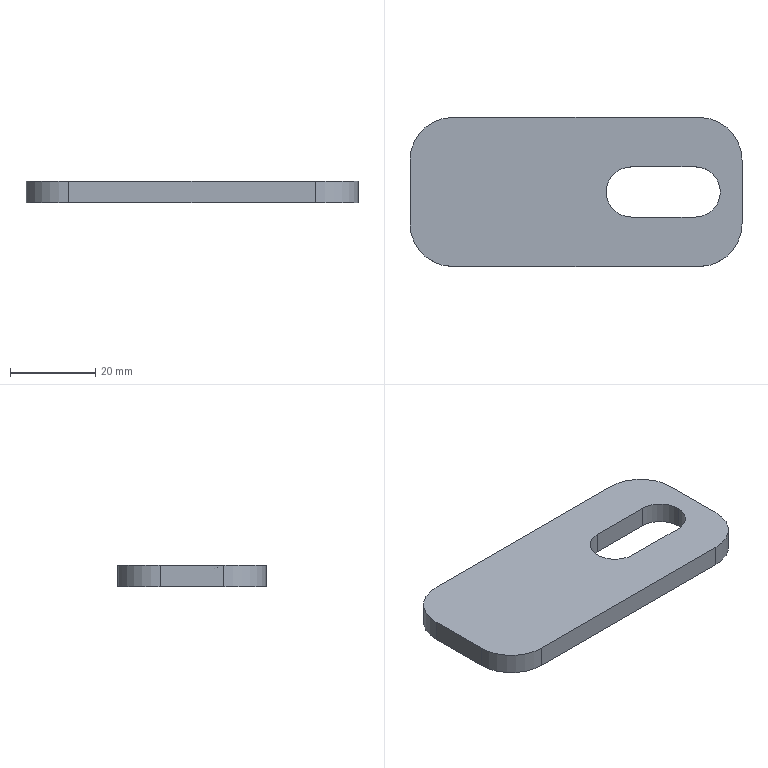Part | SolidWorks | features Fillet 1, FlatPattern 1, SMBaseFlange 1, SheetMetal 1 | 1 solid | 15 faces | box 78 x 35 x 5 mm | volume 11789 mm3 | plane 8 | cylinder 7 | commonest cylinder face diameters 20 x4 11.8 x3
STEP:
#1=CARTESIAN_POINT('',(72.9,-17.5,-5.));
#2=VERTEX_POINT('',#1);
#3=CARTESIAN_POINT('',(67.,-11.6,-5.));
#4=VERTEX_POINT('',#3);
#5=CARTESIAN_POINT('',(67.,-17.5,-5.));
#6=DIRECTION('',(0.,0.,1.));
#7=DIRECTION('',(1.,0.,0.));
#8=AXIS2_PLACEMENT_3D('',#5,#6,#7);
#9=CIRCLE('',#8,5.9);
#10=EDGE_CURVE('',#2,#4,#9,.T.);
#11=ORIENTED_EDGE('',*,*,#10,.F.);
#12=CARTESIAN_POINT('',(72.9,-17.5,0.));
#13=VERTEX_POINT('',#12);
#14=CARTESIAN_POINT('',(72.9,-17.5,-5.));
#15=DIRECTION('',(0.,0.,1.));
#16=VECTOR('',#15,1000.);
#17=LINE('',#14,#16);
#18=EDGE_CURVE('',#2,#13,#17,.T.);
#19=ORIENTED_EDGE('',*,*,#18,.T.);
#20=CARTESIAN_POINT('',(67.,-11.6,0.));
#21=VERTEX_POINT('',#20);
#22=CARTESIAN_POINT('',(67.,-17.5,0.));
#23=DIRECTION('',(0.,0.,1.));
#24=DIRECTION('',(1.,0.,0.));
#25=AXIS2_PLACEMENT_3D('',#22,#23,#24);
#26=CIRCLE('',#25,5.9);
#27=EDGE_CURVE('',#13,#21,#26,.T.);
#28=ORIENTED_EDGE('',*,*,#27,.T.);
#29=CARTESIAN_POINT('',(67.,-11.6,-5.));
#30=DIRECTION('',(0.,0.,1.));
#31=VECTOR('',#30,1000.);
#32=LINE('',#29,#31);
#33=EDGE_CURVE('',#4,#21,#32,.T.);
#34=ORIENTED_EDGE('',*,*,#33,.F.);
#35=EDGE_LOOP('',(#11,#19,#28,#34));
#36=FACE_OUTER_BOUND('',#35,.T.);
#37=CARTESIAN_POINT('',(67.,-17.5,-5.));
#38=DIRECTION('',(0.,0.,1.));
#39=DIRECTION('',(1.,0.,0.));
#40=AXIS2_PLACEMENT_3D('',#37,#38,#39);
#41=CYLINDRICAL_SURFACE('',#40,5.9);
#42=ADVANCED_FACE('',(#36),#41,.F.);
#43=CARTESIAN_POINT('',(0.,-10.,-5.));
#44=VERTEX_POINT('',#43);
#45=CARTESIAN_POINT('',(0.,-25.,-5.));
#46=VERTEX_POINT('',#45);
#47=CARTESIAN_POINT('',(0.,0.,-5.));
#48=DIRECTION('',(0.,-1.,0.));
#49=VECTOR('',#48,1000.);
#50=LINE('',#47,#49);
#51=EDGE_CURVE('',#44,#46,#50,.T.);
#52=ORIENTED_EDGE('',*,*,#51,.T.);
#53=CARTESIAN_POINT('',(0.,-25.,0.));
#54=VERTEX_POINT('',#53);
#55=CARTESIAN_POINT('',(0.,-25.,-5.));
#56=DIRECTION('',(0.,0.,1.));
#57=VECTOR('',#56,1000.);
#58=LINE('',#55,#57);
#59=EDGE_CURVE('',#46,#54,#58,.T.);
#60=ORIENTED_EDGE('',*,*,#59,.T.);
#61=CARTESIAN_POINT('',(0.,-10.,0.));
#62=VERTEX_POINT('',#61);
#63=CARTESIAN_POINT('',(0.,0.,0.));
#64=DIRECTION('',(0.,-1.,0.));
#65=VECTOR('',#64,1000.);
#66=LINE('',#63,#65);
#67=EDGE_CURVE('',#62,#54,#66,.T.);
#68=ORIENTED_EDGE('',*,*,#67,.F.);
#69=CARTESIAN_POINT('',(0.,-10.,-5.));
#70=DIRECTION('',(0.,0.,-1.));
#71=VECTOR('',#70,1000.);
#72=LINE('',#69,#71);
#73=EDGE_CURVE('',#62,#44,#72,.T.);
#74=ORIENTED_EDGE('',*,*,#73,.T.);
#75=EDGE_LOOP('',(#52,#60,#68,#74));
#76=FACE_OUTER_BOUND('',#75,.T.);
#77=CARTESIAN_POINT('',(0.,0.,-5.));
#78=DIRECTION('',(-1.,0.,0.));
#79=DIRECTION('',(0.,-1.,0.));
#80=AXIS2_PLACEMENT_3D('',#77,#78,#79);
#81=PLANE('',#80);
#82=ADVANCED_FACE('',(#76),#81,.T.);
#83=CARTESIAN_POINT('',(68.,0.,0.));
#84=VERTEX_POINT('',#83);
#85=CARTESIAN_POINT('',(10.,0.,0.));
#86=VERTEX_POINT('',#85);
#87=CARTESIAN_POINT('',(0.,0.,0.));
#88=DIRECTION('',(-1.,0.,0.));
#89=VECTOR('',#88,1000.);
#90=LINE('',#87,#89);
#91=EDGE_CURVE('',#84,#86,#90,.T.);
#92=ORIENTED_EDGE('',*,*,#91,.F.);
#93=CARTESIAN_POINT('',(68.,0.,-5.));
#94=VERTEX_POINT('',#93);
#95=CARTESIAN_POINT('',(68.,0.,-5.));
#96=DIRECTION('',(0.,0.,-1.));
#97=VECTOR('',#96,1000.);
#98=LINE('',#95,#97);
#99=EDGE_CURVE('',#84,#94,#98,.T.);
#100=ORIENTED_EDGE('',*,*,#99,.T.);
#101=CARTESIAN_POINT('',(10.,0.,-5.));
#102=VERTEX_POINT('',#101);
#103=CARTESIAN_POINT('',(0.,0.,-5.));
#104=DIRECTION('',(-1.,0.,0.));
#105=VECTOR('',#104,1000.);
#106=LINE('',#103,#105);
#107=EDGE_CURVE('',#94,#102,#106,.T.);
#108=ORIENTED_EDGE('',*,*,#107,.T.);
#109=CARTESIAN_POINT('',(10.,0.,-5.));
#110=DIRECTION('',(0.,0.,1.));
#111=VECTOR('',#110,1000.);
#112=LINE('',#109,#111);
#113=EDGE_CURVE('',#102,#86,#112,.T.);
#114=ORIENTED_EDGE('',*,*,#113,.T.);
#115=EDGE_LOOP('',(#92,#100,#108,#114));
#116=FACE_OUTER_BOUND('',#115,.T.);
#117=CARTESIAN_POINT('',(0.,0.,-5.));
#118=DIRECTION('',(0.,1.,0.));
#119=DIRECTION('',(0.,0.,1.));
#120=AXIS2_PLACEMENT_3D('',#117,#118,#119);
#121=PLANE('',#120);
#122=ADVANCED_FACE('',(#116),#121,.T.);
#123=CARTESIAN_POINT('',(78.,-25.,-5.));
#124=VERTEX_POINT('',#123);
#125=CARTESIAN_POINT('',(78.,-10.,-5.));
#126=VERTEX_POINT('',#125);
#127=CARTESIAN_POINT('',(78.,0.,-5.));
#128=DIRECTION('',(0.,1.,0.));
#129=VECTOR('',#128,1000.);
#130=LINE('',#127,#129);
#131=EDGE_CURVE('',#124,#126,#130,.T.);
#132=ORIENTED_EDGE('',*,*,#131,.T.);
#133=CARTESIAN_POINT('',(78.,-10.,0.));
#134=VERTEX_POINT('',#133);
#135=CARTESIAN_POINT('',(78.,-10.,-5.));
#136=DIRECTION('',(0.,0.,1.));
#137=VECTOR('',#136,1000.);
#138=LINE('',#135,#137);
#139=EDGE_CURVE('',#126,#134,#138,.T.);
#140=ORIENTED_EDGE('',*,*,#139,.T.);
#141=CARTESIAN_POINT('',(78.,-25.,0.));
#142=VERTEX_POINT('',#141);
#143=CARTESIAN_POINT('',(78.,0.,0.));
#144=DIRECTION('',(0.,1.,0.));
#145=VECTOR('',#144,1000.);
#146=LINE('',#143,#145);
#147=EDGE_CURVE('',#142,#134,#146,.T.);
#148=ORIENTED_EDGE('',*,*,#147,.F.);
#149=CARTESIAN_POINT('',(78.,-25.,-5.));
#150=DIRECTION('',(0.,0.,-1.));
#151=VECTOR('',#150,1000.);
#152=LINE('',#149,#151);
#153=EDGE_CURVE('',#142,#124,#152,.T.);
#154=ORIENTED_EDGE('',*,*,#153,.T.);
#155=EDGE_LOOP('',(#132,#140,#148,#154));
#156=FACE_OUTER_BOUND('',#155,.T.);
#157=CARTESIAN_POINT('',(78.,0.,-5.));
#158=DIRECTION('',(1.,0.,0.));
#159=DIRECTION('',(0.,0.,-1.));
#160=AXIS2_PLACEMENT_3D('',#157,#158,#159);
#161=PLANE('',#160);
#162=ADVANCED_FACE('',(#156),#161,.T.);
#163=CARTESIAN_POINT('',(10.,-35.,-5.));
#164=VERTEX_POINT('',#163);
#165=CARTESIAN_POINT('',(68.,-35.,-5.));
#166=VERTEX_POINT('',#165);
#167=CARTESIAN_POINT('',(0.,-35.,-5.));
#168=DIRECTION('',(1.,0.,0.));
#169=VECTOR('',#168,1000.);
#170=LINE('',#167,#169);
#171=EDGE_CURVE('',#164,#166,#170,.T.);
#172=ORIENTED_EDGE('',*,*,#171,.T.);
#173=CARTESIAN_POINT('',(68.,-35.,0.));
#174=VERTEX_POINT('',#173);
#175=CARTESIAN_POINT('',(68.,-35.,-5.));
#176=DIRECTION('',(0.,0.,1.));
#177=VECTOR('',#176,1000.);
#178=LINE('',#175,#177);
#179=EDGE_CURVE('',#166,#174,#178,.T.);
#180=ORIENTED_EDGE('',*,*,#179,.T.);
#181=CARTESIAN_POINT('',(10.,-35.,0.));
#182=VERTEX_POINT('',#181);
#183=CARTESIAN_POINT('',(0.,-35.,0.));
#184=DIRECTION('',(1.,0.,0.));
#185=VECTOR('',#184,1000.);
#186=LINE('',#183,#185);
#187=EDGE_CURVE('',#182,#174,#186,.T.);
#188=ORIENTED_EDGE('',*,*,#187,.F.);
#189=CARTESIAN_POINT('',(10.,-35.,-5.));
#190=DIRECTION('',(0.,0.,-1.));
#191=VECTOR('',#190,1000.);
#192=LINE('',#189,#191);
#193=EDGE_CURVE('',#182,#164,#192,.T.);
#194=ORIENTED_EDGE('',*,*,#193,.T.);
#195=EDGE_LOOP('',(#172,#180,#188,#194));
#196=FACE_OUTER_BOUND('',#195,.T.);
#197=CARTESIAN_POINT('',(0.,-35.,-5.));
#198=DIRECTION('',(0.,-1.,0.));
#199=DIRECTION('',(0.,0.,-1.));
#200=AXIS2_PLACEMENT_3D('',#197,#198,#199);
#201=PLANE('',#200);
#202=ADVANCED_FACE('',(#196),#201,.T.);
#203=CARTESIAN_POINT('',(52.,-23.4,-5.));
#204=VERTEX_POINT('',#203);
#205=CARTESIAN_POINT('',(67.,-23.4,-5.));
#206=VERTEX_POINT('',#205);
#207=CARTESIAN_POINT('',(67.,-23.4,-5.));
#208=DIRECTION('',(1.,0.,0.));
#209=VECTOR('',#208,1000.);
#210=LINE('',#207,#209);
#211=EDGE_CURVE('',#204,#206,#210,.T.);
#212=ORIENTED_EDGE('',*,*,#211,.T.);
#213=CARTESIAN_POINT('',(67.,-17.5,-5.));
#214=DIRECTION('',(0.,0.,1.));
#215=DIRECTION('',(1.,0.,0.));
#216=AXIS2_PLACEMENT_3D('',#213,#214,#215);
#217=CIRCLE('',#216,5.9);
#218=EDGE_CURVE('',#206,#2,#217,.T.);
#219=ORIENTED_EDGE('',*,*,#218,.T.);
#220=ORIENTED_EDGE('',*,*,#10,.T.);
#221=CARTESIAN_POINT('',(52.,-11.6,-5.));
#222=VERTEX_POINT('',#221);
#223=CARTESIAN_POINT('',(67.,-11.6,-5.));
#224=DIRECTION('',(-1.,0.,0.));
#225=VECTOR('',#224,1000.);
#226=LINE('',#223,#225);
#227=EDGE_CURVE('',#4,#222,#226,.T.);
#228=ORIENTED_EDGE('',*,*,#227,.T.);
#229=CARTESIAN_POINT('',(52.,-17.5,-5.));
#230=DIRECTION('',(0.,0.,1.));
#231=DIRECTION('',(1.,0.,0.));
#232=AXIS2_PLACEMENT_3D('',#229,#230,#231);
#233=CIRCLE('',#232,5.9);
#234=EDGE_CURVE('',#222,#204,#233,.T.);
#235=ORIENTED_EDGE('',*,*,#234,.T.);
#236=EDGE_LOOP('',(#212,#219,#220,#228,#235));
#237=FACE_BOUND('',#236,.T.);
#238=ORIENTED_EDGE('',*,*,#107,.F.);
#239=CARTESIAN_POINT('',(68.,-10.,-5.));
#240=DIRECTION('',(0.,0.,-1.));
#241=DIRECTION('',(1.,0.,0.));
#242=AXIS2_PLACEMENT_3D('',#239,#240,#241);
#243=CIRCLE('',#242,10.);
#244=EDGE_CURVE('',#94,#126,#243,.T.);
#245=ORIENTED_EDGE('',*,*,#244,.T.);
#246=ORIENTED_EDGE('',*,*,#131,.F.);
#247=CARTESIAN_POINT('',(68.,-25.,-5.));
#248=DIRECTION('',(0.,0.,-1.));
#249=DIRECTION('',(1.,0.,0.));
#250=AXIS2_PLACEMENT_3D('',#247,#248,#249);
#251=CIRCLE('',#250,10.);
#252=EDGE_CURVE('',#124,#166,#251,.T.);
#253=ORIENTED_EDGE('',*,*,#252,.T.);
#254=ORIENTED_EDGE('',*,*,#171,.F.);
#255=CARTESIAN_POINT('',(10.,-25.,-5.));
#256=DIRECTION('',(0.,0.,-1.));
#257=DIRECTION('',(1.,0.,0.));
#258=AXIS2_PLACEMENT_3D('',#255,#256,#257);
#259=CIRCLE('',#258,10.);
#260=EDGE_CURVE('',#164,#46,#259,.T.);
#261=ORIENTED_EDGE('',*,*,#260,.T.);
#262=ORIENTED_EDGE('',*,*,#51,.F.);
#263=CARTESIAN_POINT('',(10.,-10.,-5.));
#264=DIRECTION('',(0.,0.,-1.));
#265=DIRECTION('',(1.,0.,0.));
#266=AXIS2_PLACEMENT_3D('',#263,#264,#265);
#267=CIRCLE('',#266,10.);
#268=EDGE_CURVE('',#44,#102,#267,.T.);
#269=ORIENTED_EDGE('',*,*,#268,.T.);
#270=EDGE_LOOP('',(#238,#245,#246,#253,#254,#261,#262,#269));
#271=FACE_OUTER_BOUND('',#270,.T.);
#272=CARTESIAN_POINT('',(0.,0.,-5.));
#273=DIRECTION('',(0.,0.,1.));
#274=DIRECTION('',(1.,0.,0.));
#275=AXIS2_PLACEMENT_3D('',#272,#273,#274);
#276=PLANE('',#275);
#277=ADVANCED_FACE('',(#237,#271),#276,.F.);
#278=CARTESIAN_POINT('',(67.,-23.4,0.));
#279=VERTEX_POINT('',#278);
#280=CARTESIAN_POINT('',(67.,-17.5,0.));
#281=DIRECTION('',(0.,0.,1.));
#282=DIRECTION('',(1.,0.,0.));
#283=AXIS2_PLACEMENT_3D('',#280,#281,#282);
#284=CIRCLE('',#283,5.9);
#285=EDGE_CURVE('',#279,#13,#284,.T.);
#286=ORIENTED_EDGE('',*,*,#285,.F.);
#287=CARTESIAN_POINT('',(52.,-23.4,0.));
#288=VERTEX_POINT('',#287);
#289=CARTESIAN_POINT('',(67.,-23.4,0.));
#290=DIRECTION('',(1.,0.,0.));
#291=VECTOR('',#290,1000.);
#292=LINE('',#289,#291);
#293=EDGE_CURVE('',#288,#279,#292,.T.);
#294=ORIENTED_EDGE('',*,*,#293,.F.);
#295=CARTESIAN_POINT('',(52.,-11.6,0.));
#296=VERTEX_POINT('',#295);
#297=CARTESIAN_POINT('',(52.,-17.5,0.));
#298=DIRECTION('',(0.,0.,1.));
#299=DIRECTION('',(1.,0.,0.));
#300=AXIS2_PLACEMENT_3D('',#297,#298,#299);
#301=CIRCLE('',#300,5.9);
#302=EDGE_CURVE('',#296,#288,#301,.T.);
#303=ORIENTED_EDGE('',*,*,#302,.F.);
#304=CARTESIAN_POINT('',(67.,-11.6,0.));
#305=DIRECTION('',(-1.,0.,0.));
#306=VECTOR('',#305,1000.);
#307=LINE('',#304,#306);
#308=EDGE_CURVE('',#21,#296,#307,.T.);
#309=ORIENTED_EDGE('',*,*,#308,.F.);
#310=ORIENTED_EDGE('',*,*,#27,.F.);
#311=EDGE_LOOP('',(#286,#294,#303,#309,#310));
#312=FACE_BOUND('',#311,.T.);
#313=ORIENTED_EDGE('',*,*,#147,.T.);
#314=CARTESIAN_POINT('',(68.,-10.,0.));
#315=DIRECTION('',(0.,0.,1.));
#316=DIRECTION('',(1.,0.,0.));
#317=AXIS2_PLACEMENT_3D('',#314,#315,#316);
#318=CIRCLE('',#317,10.);
#319=EDGE_CURVE('',#134,#84,#318,.T.);
#320=ORIENTED_EDGE('',*,*,#319,.T.);
#321=ORIENTED_EDGE('',*,*,#91,.T.);
#322=CARTESIAN_POINT('',(10.,-10.,0.));
#323=DIRECTION('',(0.,0.,1.));
#324=DIRECTION('',(1.,0.,0.));
#325=AXIS2_PLACEMENT_3D('',#322,#323,#324);
#326=CIRCLE('',#325,10.);
#327=EDGE_CURVE('',#86,#62,#326,.T.);
#328=ORIENTED_EDGE('',*,*,#327,.T.);
#329=ORIENTED_EDGE('',*,*,#67,.T.);
#330=CARTESIAN_POINT('',(10.,-25.,0.));
#331=DIRECTION('',(0.,0.,1.));
#332=DIRECTION('',(1.,0.,0.));
#333=AXIS2_PLACEMENT_3D('',#330,#331,#332);
#334=CIRCLE('',#333,10.);
#335=EDGE_CURVE('',#54,#182,#334,.T.);
#336=ORIENTED_EDGE('',*,*,#335,.T.);
#337=ORIENTED_EDGE('',*,*,#187,.T.);
#338=CARTESIAN_POINT('',(68.,-25.,0.));
#339=DIRECTION('',(0.,0.,1.));
#340=DIRECTION('',(1.,0.,0.));
#341=AXIS2_PLACEMENT_3D('',#338,#339,#340);
#342=CIRCLE('',#341,10.);
#343=EDGE_CURVE('',#174,#142,#342,.T.);
#344=ORIENTED_EDGE('',*,*,#343,.T.);
#345=EDGE_LOOP('',(#313,#320,#321,#328,#329,#336,#337,#344));
#346=FACE_OUTER_BOUND('',#345,.T.);
#347=CARTESIAN_POINT('',(0.,0.,0.));
#348=DIRECTION('',(0.,0.,1.));
#349=DIRECTION('',(1.,0.,0.));
#350=AXIS2_PLACEMENT_3D('',#347,#348,#349);
#351=PLANE('',#350);
#352=ADVANCED_FACE('',(#312,#346),#351,.T.);
#353=ORIENTED_EDGE('',*,*,#18,.F.);
#354=ORIENTED_EDGE('',*,*,#218,.F.);
#355=CARTESIAN_POINT('',(67.,-23.4,-5.));
#356=DIRECTION('',(0.,0.,1.));
#357=VECTOR('',#356,1000.);
#358=LINE('',#355,#357);
#359=EDGE_CURVE('',#206,#279,#358,.T.);
#360=ORIENTED_EDGE('',*,*,#359,.T.);
#361=ORIENTED_EDGE('',*,*,#285,.T.);
#362=EDGE_LOOP('',(#353,#354,#360,#361));
#363=FACE_OUTER_BOUND('',#362,.T.);
#364=CARTESIAN_POINT('',(67.,-17.5,-5.));
#365=DIRECTION('',(0.,0.,1.));
#366=DIRECTION('',(1.,0.,0.));
#367=AXIS2_PLACEMENT_3D('',#364,#365,#366);
#368=CYLINDRICAL_SURFACE('',#367,5.9);
#369=ADVANCED_FACE('',(#363),#368,.F.);
#370=ORIENTED_EDGE('',*,*,#293,.T.);
#371=ORIENTED_EDGE('',*,*,#359,.F.);
#372=ORIENTED_EDGE('',*,*,#211,.F.);
#373=CARTESIAN_POINT('',(52.,-23.4,-5.));
#374=DIRECTION('',(0.,0.,1.));
#375=VECTOR('',#374,1000.);
#376=LINE('',#373,#375);
#377=EDGE_CURVE('',#204,#288,#376,.T.);
#378=ORIENTED_EDGE('',*,*,#377,.T.);
#379=EDGE_LOOP('',(#370,#371,#372,#378));
#380=FACE_OUTER_BOUND('',#379,.T.);
#381=CARTESIAN_POINT('',(67.,-23.4,-5.));
#382=DIRECTION('',(0.,-1.,0.));
#383=DIRECTION('',(0.,0.,-1.));
#384=AXIS2_PLACEMENT_3D('',#381,#382,#383);
#385=PLANE('',#384);
#386=ADVANCED_FACE('',(#380),#385,.F.);
#387=ORIENTED_EDGE('',*,*,#302,.T.);
#388=ORIENTED_EDGE('',*,*,#377,.F.);
#389=ORIENTED_EDGE('',*,*,#234,.F.);
#390=CARTESIAN_POINT('',(52.,-11.6,-5.));
#391=DIRECTION('',(0.,0.,1.));
#392=VECTOR('',#391,1000.);
#393=LINE('',#390,#392);
#394=EDGE_CURVE('',#222,#296,#393,.T.);
#395=ORIENTED_EDGE('',*,*,#394,.T.);
#396=EDGE_LOOP('',(#387,#388,#389,#395));
#397=FACE_OUTER_BOUND('',#396,.T.);
#398=CARTESIAN_POINT('',(52.,-17.5,-5.));
#399=DIRECTION('',(0.,0.,1.));
#400=DIRECTION('',(1.,0.,0.));
#401=AXIS2_PLACEMENT_3D('',#398,#399,#400);
#402=CYLINDRICAL_SURFACE('',#401,5.9);
#403=ADVANCED_FACE('',(#397),#402,.F.);
#404=ORIENTED_EDGE('',*,*,#308,.T.);
#405=ORIENTED_EDGE('',*,*,#394,.F.);
#406=ORIENTED_EDGE('',*,*,#227,.F.);
#407=ORIENTED_EDGE('',*,*,#33,.T.);
#408=EDGE_LOOP('',(#404,#405,#406,#407));
#409=FACE_OUTER_BOUND('',#408,.T.);
#410=CARTESIAN_POINT('',(67.,-11.6,-5.));
#411=DIRECTION('',(0.,1.,0.));
#412=DIRECTION('',(-1.,0.,0.));
#413=AXIS2_PLACEMENT_3D('',#410,#411,#412);
#414=PLANE('',#413);
#415=ADVANCED_FACE('',(#409),#414,.F.);
#416=ORIENTED_EDGE('',*,*,#244,.F.);
#417=ORIENTED_EDGE('',*,*,#99,.F.);
#418=ORIENTED_EDGE('',*,*,#319,.F.);
#419=ORIENTED_EDGE('',*,*,#139,.F.);
#420=EDGE_LOOP('',(#416,#417,#418,#419));
#421=FACE_OUTER_BOUND('',#420,.T.);
#422=CARTESIAN_POINT('',(68.,-10.,-5.));
#423=DIRECTION('',(0.,0.,1.));
#424=DIRECTION('',(1.,0.,0.));
#425=AXIS2_PLACEMENT_3D('',#422,#423,#424);
#426=CYLINDRICAL_SURFACE('',#425,10.);
#427=ADVANCED_FACE('',(#421),#426,.T.);
#428=ORIENTED_EDGE('',*,*,#252,.F.);
#429=ORIENTED_EDGE('',*,*,#153,.F.);
#430=ORIENTED_EDGE('',*,*,#343,.F.);
#431=ORIENTED_EDGE('',*,*,#179,.F.);
#432=EDGE_LOOP('',(#428,#429,#430,#431));
#433=FACE_OUTER_BOUND('',#432,.T.);
#434=CARTESIAN_POINT('',(68.,-25.,-5.));
#435=DIRECTION('',(0.,0.,1.));
#436=DIRECTION('',(1.,0.,0.));
#437=AXIS2_PLACEMENT_3D('',#434,#435,#436);
#438=CYLINDRICAL_SURFACE('',#437,10.);
#439=ADVANCED_FACE('',(#433),#438,.T.);
#440=ORIENTED_EDGE('',*,*,#260,.F.);
#441=ORIENTED_EDGE('',*,*,#193,.F.);
#442=ORIENTED_EDGE('',*,*,#335,.F.);
#443=ORIENTED_EDGE('',*,*,#59,.F.);
#444=EDGE_LOOP('',(#440,#441,#442,#443));
#445=FACE_OUTER_BOUND('',#444,.T.);
#446=CARTESIAN_POINT('',(10.,-25.,-5.));
#447=DIRECTION('',(0.,0.,1.));
#448=DIRECTION('',(1.,0.,0.));
#449=AXIS2_PLACEMENT_3D('',#446,#447,#448);
#450=CYLINDRICAL_SURFACE('',#449,10.);
#451=ADVANCED_FACE('',(#445),#450,.T.);
#452=ORIENTED_EDGE('',*,*,#268,.F.);
#453=ORIENTED_EDGE('',*,*,#73,.F.);
#454=ORIENTED_EDGE('',*,*,#327,.F.);
#455=ORIENTED_EDGE('',*,*,#113,.F.);
#456=EDGE_LOOP('',(#452,#453,#454,#455));
#457=FACE_OUTER_BOUND('',#456,.T.);
#458=CARTESIAN_POINT('',(10.,-10.,-5.));
#459=DIRECTION('',(0.,0.,1.));
#460=DIRECTION('',(1.,0.,0.));
#461=AXIS2_PLACEMENT_3D('',#458,#459,#460);
#462=CYLINDRICAL_SURFACE('',#461,10.);
#463=ADVANCED_FACE('',(#457),#462,.T.);
#464=CLOSED_SHELL('',(#42,#82,#122,#162,#202,#277,#352,#369,#386,#403,#415,#427,#439,#451,#463));
#465=MANIFOLD_SOLID_BREP('',#464);
#466=CARTESIAN_POINT('',(0.,0.,0.));
#467=DIRECTION('',(0.,0.,1.));
#468=DIRECTION('',(1.,0.,0.));
#469=AXIS2_PLACEMENT_3D('',#466,#467,#468);
#470=(LENGTH_UNIT()NAMED_UNIT(*)SI_UNIT(.MILLI.,.METRE.));
#471=UNCERTAINTY_MEASURE_WITH_UNIT(LENGTH_MEASURE(0.00001),#470,'','');
#472=(NAMED_UNIT(*)PLANE_ANGLE_UNIT()SI_UNIT($,.RADIAN.));
#473=(NAMED_UNIT(*)SI_UNIT($,.STERADIAN.)SOLID_ANGLE_UNIT());
#474=(GEOMETRIC_REPRESENTATION_CONTEXT(3)GLOBAL_UNCERTAINTY_ASSIGNED_CONTEXT((#471))GLOBAL_UNIT_ASSIGNED_CONTEXT((#470,#472,#473))REPRESENTATION_CONTEXT('',''));
#475=ADVANCED_BREP_SHAPE_REPRESENTATION('',(#465,#469),#474);